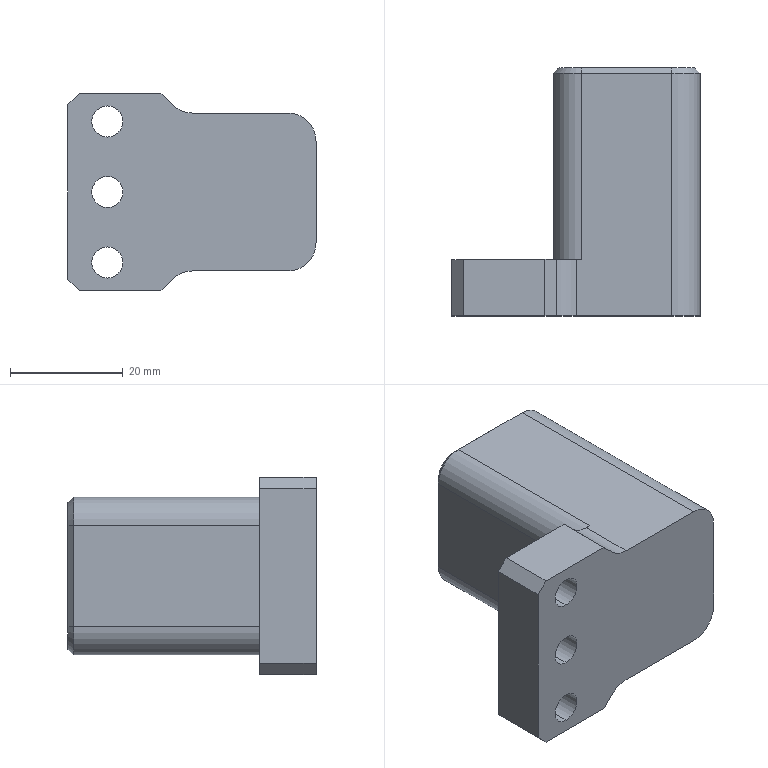Part | SolidWorks | features Chamfer 3, Fillet 2, HoleWzd 2, Extrusion 1, ICE 1 | 1 solid | 34 faces | box 44 x 44 x 35 mm | volume 36722 mm3 | plane 18 | cylinder 12 | cone 4 | commonest cylinder face diameters 5.5 x6 10 x6
STEP:
#1=CARTESIAN_POINT('',(-37.,0.,-15.25));
#2=VERTEX_POINT('',#1);
#3=CARTESIAN_POINT('',(-37.,0.,-9.75));
#4=VERTEX_POINT('',#3);
#5=CARTESIAN_POINT('',(-37.,0.,-12.5));
#6=DIRECTION('',(0.,1.,0.));
#7=DIRECTION('',(0.,0.,1.));
#8=AXIS2_PLACEMENT_3D('',#5,#6,#7);
#9=CIRCLE('',#8,2.75);
#10=EDGE_CURVE('',#2,#4,#9,.T.);
#11=ORIENTED_EDGE('',*,*,#10,.F.);
#12=CARTESIAN_POINT('',(-37.,10.,-15.25));
#13=VERTEX_POINT('',#12);
#14=CARTESIAN_POINT('',(-37.,10.,-15.25));
#15=DIRECTION('',(0.,1.,0.));
#16=VECTOR('',#15,1000.);
#17=LINE('',#14,#16);
#18=EDGE_CURVE('',#2,#13,#17,.T.);
#19=ORIENTED_EDGE('',*,*,#18,.T.);
#20=CARTESIAN_POINT('',(-37.,10.,-9.75));
#21=VERTEX_POINT('',#20);
#22=CARTESIAN_POINT('',(-37.,10.,-12.5));
#23=DIRECTION('',(0.,1.,0.));
#24=DIRECTION('',(0.,0.,1.));
#25=AXIS2_PLACEMENT_3D('',#22,#23,#24);
#26=CIRCLE('',#25,2.75);
#27=EDGE_CURVE('',#13,#21,#26,.T.);
#28=ORIENTED_EDGE('',*,*,#27,.T.);
#29=CARTESIAN_POINT('',(-37.,10.,-9.75));
#30=DIRECTION('',(0.,1.,0.));
#31=VECTOR('',#30,1000.);
#32=LINE('',#29,#31);
#33=EDGE_CURVE('',#4,#21,#32,.T.);
#34=ORIENTED_EDGE('',*,*,#33,.F.);
#35=EDGE_LOOP('',(#11,#19,#28,#34));
#36=FACE_OUTER_BOUND('',#35,.T.);
#37=CARTESIAN_POINT('',(-37.,10.,-12.5));
#38=DIRECTION('',(0.,1.,0.));
#39=DIRECTION('',(0.,0.,1.));
#40=AXIS2_PLACEMENT_3D('',#37,#38,#39);
#41=CYLINDRICAL_SURFACE('',#40,2.75);
#42=ADVANCED_FACE('',(#36),#41,.F.);
#43=CARTESIAN_POINT('',(-37.,0.,9.75));
#44=VERTEX_POINT('',#43);
#45=CARTESIAN_POINT('',(-37.,0.,15.25));
#46=VERTEX_POINT('',#45);
#47=CARTESIAN_POINT('',(-37.,0.,12.5));
#48=DIRECTION('',(0.,1.,0.));
#49=DIRECTION('',(0.,0.,1.));
#50=AXIS2_PLACEMENT_3D('',#47,#48,#49);
#51=CIRCLE('',#50,2.75);
#52=EDGE_CURVE('',#44,#46,#51,.T.);
#53=ORIENTED_EDGE('',*,*,#52,.F.);
#54=CARTESIAN_POINT('',(-37.,10.,9.75));
#55=VERTEX_POINT('',#54);
#56=CARTESIAN_POINT('',(-37.,10.,9.75));
#57=DIRECTION('',(0.,1.,0.));
#58=VECTOR('',#57,1000.);
#59=LINE('',#56,#58);
#60=EDGE_CURVE('',#44,#55,#59,.T.);
#61=ORIENTED_EDGE('',*,*,#60,.T.);
#62=CARTESIAN_POINT('',(-37.,10.,15.25));
#63=VERTEX_POINT('',#62);
#64=CARTESIAN_POINT('',(-37.,10.,12.5));
#65=DIRECTION('',(0.,1.,0.));
#66=DIRECTION('',(0.,0.,1.));
#67=AXIS2_PLACEMENT_3D('',#64,#65,#66);
#68=CIRCLE('',#67,2.75);
#69=EDGE_CURVE('',#55,#63,#68,.T.);
#70=ORIENTED_EDGE('',*,*,#69,.T.);
#71=CARTESIAN_POINT('',(-37.,10.,15.25));
#72=DIRECTION('',(0.,1.,0.));
#73=VECTOR('',#72,1000.);
#74=LINE('',#71,#73);
#75=EDGE_CURVE('',#46,#63,#74,.T.);
#76=ORIENTED_EDGE('',*,*,#75,.F.);
#77=EDGE_LOOP('',(#53,#61,#70,#76));
#78=FACE_OUTER_BOUND('',#77,.T.);
#79=CARTESIAN_POINT('',(-37.,10.,12.5));
#80=DIRECTION('',(0.,1.,0.));
#81=DIRECTION('',(0.,0.,1.));
#82=AXIS2_PLACEMENT_3D('',#79,#80,#81);
#83=CYLINDRICAL_SURFACE('',#82,2.75);
#84=ADVANCED_FACE('',(#78),#83,.F.);
#85=CARTESIAN_POINT('',(-37.,0.,-2.75));
#86=VERTEX_POINT('',#85);
#87=CARTESIAN_POINT('',(-37.,0.,2.75));
#88=VERTEX_POINT('',#87);
#89=CARTESIAN_POINT('',(-37.,0.,0.));
#90=DIRECTION('',(0.,1.,0.));
#91=DIRECTION('',(0.,0.,1.));
#92=AXIS2_PLACEMENT_3D('',#89,#90,#91);
#93=CIRCLE('',#92,2.75);
#94=EDGE_CURVE('',#86,#88,#93,.T.);
#95=ORIENTED_EDGE('',*,*,#94,.F.);
#96=CARTESIAN_POINT('',(-37.,10.,-2.75));
#97=VERTEX_POINT('',#96);
#98=CARTESIAN_POINT('',(-37.,10.,-2.75));
#99=DIRECTION('',(0.,1.,0.));
#100=VECTOR('',#99,1000.);
#101=LINE('',#98,#100);
#102=EDGE_CURVE('',#86,#97,#101,.T.);
#103=ORIENTED_EDGE('',*,*,#102,.T.);
#104=CARTESIAN_POINT('',(-37.,10.,2.75));
#105=VERTEX_POINT('',#104);
#106=CARTESIAN_POINT('',(-37.,10.,0.));
#107=DIRECTION('',(0.,1.,0.));
#108=DIRECTION('',(0.,0.,1.));
#109=AXIS2_PLACEMENT_3D('',#106,#107,#108);
#110=CIRCLE('',#109,2.75);
#111=EDGE_CURVE('',#97,#105,#110,.T.);
#112=ORIENTED_EDGE('',*,*,#111,.T.);
#113=CARTESIAN_POINT('',(-37.,10.,2.75));
#114=DIRECTION('',(0.,1.,0.));
#115=VECTOR('',#114,1000.);
#116=LINE('',#113,#115);
#117=EDGE_CURVE('',#88,#105,#116,.T.);
#118=ORIENTED_EDGE('',*,*,#117,.F.);
#119=EDGE_LOOP('',(#95,#103,#112,#118));
#120=FACE_OUTER_BOUND('',#119,.T.);
#121=CARTESIAN_POINT('',(-37.,10.,0.));
#122=DIRECTION('',(0.,1.,0.));
#123=DIRECTION('',(0.,0.,1.));
#124=AXIS2_PLACEMENT_3D('',#121,#122,#123);
#125=CYLINDRICAL_SURFACE('',#124,2.75);
#126=ADVANCED_FACE('',(#120),#125,.F.);
#127=CARTESIAN_POINT('',(-37.,0.,-12.5));
#128=DIRECTION('',(0.,1.,0.));
#129=DIRECTION('',(0.,0.,1.));
#130=AXIS2_PLACEMENT_3D('',#127,#128,#129);
#131=CIRCLE('',#130,2.75);
#132=EDGE_CURVE('',#4,#2,#131,.T.);
#133=ORIENTED_EDGE('',*,*,#132,.T.);
#134=ORIENTED_EDGE('',*,*,#10,.T.);
#135=EDGE_LOOP('',(#133,#134));
#136=FACE_BOUND('',#135,.T.);
#137=CARTESIAN_POINT('',(-37.,0.,12.5));
#138=DIRECTION('',(0.,1.,0.));
#139=DIRECTION('',(0.,0.,1.));
#140=AXIS2_PLACEMENT_3D('',#137,#138,#139);
#141=CIRCLE('',#140,2.75);
#142=EDGE_CURVE('',#46,#44,#141,.T.);
#143=ORIENTED_EDGE('',*,*,#142,.T.);
#144=ORIENTED_EDGE('',*,*,#52,.T.);
#145=EDGE_LOOP('',(#143,#144));
#146=FACE_BOUND('',#145,.T.);
#147=CARTESIAN_POINT('',(-37.,0.,0.));
#148=DIRECTION('',(0.,1.,0.));
#149=DIRECTION('',(0.,0.,1.));
#150=AXIS2_PLACEMENT_3D('',#147,#148,#149);
#151=CIRCLE('',#150,2.75);
#152=EDGE_CURVE('',#88,#86,#151,.T.);
#153=ORIENTED_EDGE('',*,*,#152,.T.);
#154=ORIENTED_EDGE('',*,*,#94,.T.);
#155=EDGE_LOOP('',(#153,#154));
#156=FACE_BOUND('',#155,.T.);
#157=CARTESIAN_POINT('',(-44.,0.,15.5));
#158=VERTEX_POINT('',#157);
#159=CARTESIAN_POINT('',(-44.,0.,-15.5));
#160=VERTEX_POINT('',#159);
#161=CARTESIAN_POINT('',(-44.,0.,14.));
#162=DIRECTION('',(0.,0.,-1.));
#163=VECTOR('',#162,1000.);
#164=LINE('',#161,#163);
#165=EDGE_CURVE('',#158,#160,#164,.T.);
#166=ORIENTED_EDGE('',*,*,#165,.T.);
#167=CARTESIAN_POINT('',(-42.,0.,-17.5));
#168=VERTEX_POINT('',#167);
#169=CARTESIAN_POINT('',(-44.,0.,-15.5));
#170=DIRECTION('',(0.7071,0.,-0.7071));
#171=VECTOR('',#170,1000.);
#172=LINE('',#169,#171);
#173=EDGE_CURVE('',#160,#168,#172,.T.);
#174=ORIENTED_EDGE('',*,*,#173,.T.);
#175=CARTESIAN_POINT('',(-27.5,0.,-17.5));
#176=VERTEX_POINT('',#175);
#177=CARTESIAN_POINT('',(-44.,0.,-17.5));
#178=DIRECTION('',(1.,0.,0.));
#179=VECTOR('',#178,1000.);
#180=LINE('',#177,#179);
#181=EDGE_CURVE('',#168,#176,#180,.T.);
#182=ORIENTED_EDGE('',*,*,#181,.T.);
#183=CARTESIAN_POINT('',(-25.464,0.,-15.464));
#184=VERTEX_POINT('',#183);
#185=CARTESIAN_POINT('',(-27.5,0.,-17.5));
#186=DIRECTION('',(0.7071,0.,0.7071));
#187=VECTOR('',#186,1000.);
#188=LINE('',#185,#187);
#189=EDGE_CURVE('',#176,#184,#188,.T.);
#190=ORIENTED_EDGE('',*,*,#189,.T.);
#191=CARTESIAN_POINT('',(-21.929,0.,-14.));
#192=VERTEX_POINT('',#191);
#193=CARTESIAN_POINT('',(-21.929,0.,-19.));
#194=DIRECTION('',(0.,1.,0.));
#195=DIRECTION('',(0.,0.,1.));
#196=AXIS2_PLACEMENT_3D('',#193,#194,#195);
#197=CIRCLE('',#196,5.);
#198=EDGE_CURVE('',#184,#192,#197,.T.);
#199=ORIENTED_EDGE('',*,*,#198,.T.);
#200=CARTESIAN_POINT('',(-5.,0.,-14.));
#201=VERTEX_POINT('',#200);
#202=CARTESIAN_POINT('',(-44.,0.,-14.));
#203=DIRECTION('',(1.,0.,0.));
#204=VECTOR('',#203,1000.);
#205=LINE('',#202,#204);
#206=EDGE_CURVE('',#192,#201,#205,.T.);
#207=ORIENTED_EDGE('',*,*,#206,.T.);
#208=CARTESIAN_POINT('',(0.,0.,-9.));
#209=VERTEX_POINT('',#208);
#210=CARTESIAN_POINT('',(-5.,0.,-9.));
#211=DIRECTION('',(0.,-1.,0.));
#212=DIRECTION('',(0.,0.,1.));
#213=AXIS2_PLACEMENT_3D('',#210,#211,#212);
#214=CIRCLE('',#213,5.);
#215=EDGE_CURVE('',#201,#209,#214,.T.);
#216=ORIENTED_EDGE('',*,*,#215,.T.);
#217=CARTESIAN_POINT('',(0.,0.,9.));
#218=VERTEX_POINT('',#217);
#219=CARTESIAN_POINT('',(0.,0.,14.));
#220=DIRECTION('',(0.,0.,-1.));
#221=VECTOR('',#220,1000.);
#222=LINE('',#219,#221);
#223=EDGE_CURVE('',#218,#209,#222,.T.);
#224=ORIENTED_EDGE('',*,*,#223,.F.);
#225=CARTESIAN_POINT('',(-5.,0.,14.));
#226=VERTEX_POINT('',#225);
#227=CARTESIAN_POINT('',(-5.,0.,9.));
#228=DIRECTION('',(0.,-1.,0.));
#229=DIRECTION('',(0.,0.,1.));
#230=AXIS2_PLACEMENT_3D('',#227,#228,#229);
#231=CIRCLE('',#230,5.);
#232=EDGE_CURVE('',#218,#226,#231,.T.);
#233=ORIENTED_EDGE('',*,*,#232,.T.);
#234=CARTESIAN_POINT('',(-21.929,0.,14.));
#235=VERTEX_POINT('',#234);
#236=CARTESIAN_POINT('',(-44.,0.,14.));
#237=DIRECTION('',(1.,0.,0.));
#238=VECTOR('',#237,1000.);
#239=LINE('',#236,#238);
#240=EDGE_CURVE('',#235,#226,#239,.T.);
#241=ORIENTED_EDGE('',*,*,#240,.F.);
#242=CARTESIAN_POINT('',(-25.464,0.,15.464));
#243=VERTEX_POINT('',#242);
#244=CARTESIAN_POINT('',(-21.929,0.,19.));
#245=DIRECTION('',(0.,1.,0.));
#246=DIRECTION('',(0.,0.,1.));
#247=AXIS2_PLACEMENT_3D('',#244,#245,#246);
#248=CIRCLE('',#247,5.);
#249=EDGE_CURVE('',#235,#243,#248,.T.);
#250=ORIENTED_EDGE('',*,*,#249,.T.);
#251=CARTESIAN_POINT('',(-27.5,0.,17.5));
#252=VERTEX_POINT('',#251);
#253=CARTESIAN_POINT('',(-24.,0.,14.));
#254=DIRECTION('',(-0.7071,0.,0.7071));
#255=VECTOR('',#254,1000.);
#256=LINE('',#253,#255);
#257=EDGE_CURVE('',#243,#252,#256,.T.);
#258=ORIENTED_EDGE('',*,*,#257,.T.);
#259=CARTESIAN_POINT('',(-42.,0.,17.5));
#260=VERTEX_POINT('',#259);
#261=CARTESIAN_POINT('',(-44.,0.,17.5));
#262=DIRECTION('',(-1.,0.,0.));
#263=VECTOR('',#262,1000.);
#264=LINE('',#261,#263);
#265=EDGE_CURVE('',#252,#260,#264,.T.);
#266=ORIENTED_EDGE('',*,*,#265,.T.);
#267=CARTESIAN_POINT('',(-42.,0.,17.5));
#268=DIRECTION('',(-0.7071,0.,-0.7071));
#269=VECTOR('',#268,1000.);
#270=LINE('',#267,#269);
#271=EDGE_CURVE('',#260,#158,#270,.T.);
#272=ORIENTED_EDGE('',*,*,#271,.T.);
#273=EDGE_LOOP('',(#166,#174,#182,#190,#199,#207,#216,#224,#233,#241,#250,#258,#266,#272));
#274=FACE_OUTER_BOUND('',#273,.T.);
#275=CARTESIAN_POINT('',(-44.,0.,14.));
#276=DIRECTION('',(0.,1.,0.));
#277=DIRECTION('',(0.,0.,1.));
#278=AXIS2_PLACEMENT_3D('',#275,#276,#277);
#279=PLANE('',#278);
#280=ADVANCED_FACE('',(#136,#146,#156,#274),#279,.F.);
#281=CARTESIAN_POINT('',(0.,43.,-9.));
#282=VERTEX_POINT('',#281);
#283=CARTESIAN_POINT('',(0.,0.,-9.));
#284=DIRECTION('',(0.,1.,0.));
#285=VECTOR('',#284,1000.);
#286=LINE('',#283,#285);
#287=EDGE_CURVE('',#209,#282,#286,.T.);
#288=ORIENTED_EDGE('',*,*,#287,.T.);
#289=CARTESIAN_POINT('',(0.,43.,9.));
#290=VERTEX_POINT('',#289);
#291=CARTESIAN_POINT('',(0.,43.,14.));
#292=DIRECTION('',(0.,0.,1.));
#293=VECTOR('',#292,1000.);
#294=LINE('',#291,#293);
#295=EDGE_CURVE('',#282,#290,#294,.T.);
#296=ORIENTED_EDGE('',*,*,#295,.T.);
#297=CARTESIAN_POINT('',(0.,0.,9.));
#298=DIRECTION('',(0.,-1.,0.));
#299=VECTOR('',#298,1000.);
#300=LINE('',#297,#299);
#301=EDGE_CURVE('',#290,#218,#300,.T.);
#302=ORIENTED_EDGE('',*,*,#301,.T.);
#303=ORIENTED_EDGE('',*,*,#223,.T.);
#304=EDGE_LOOP('',(#288,#296,#302,#303));
#305=FACE_OUTER_BOUND('',#304,.T.);
#306=CARTESIAN_POINT('',(0.,0.,14.));
#307=DIRECTION('',(-1.,0.,0.));
#308=DIRECTION('',(0.,0.,1.));
#309=AXIS2_PLACEMENT_3D('',#306,#307,#308);
#310=PLANE('',#309);
#311=ADVANCED_FACE('',(#305),#310,.F.);
#312=CARTESIAN_POINT('',(-1.,44.,9.));
#313=VERTEX_POINT('',#312);
#314=CARTESIAN_POINT('',(-1.,44.,-9.));
#315=VERTEX_POINT('',#314);
#316=CARTESIAN_POINT('',(-1.,44.,14.));
#317=DIRECTION('',(0.,0.,-1.));
#318=VECTOR('',#317,1000.);
#319=LINE('',#316,#318);
#320=EDGE_CURVE('',#313,#315,#319,.T.);
#321=ORIENTED_EDGE('',*,*,#320,.T.);
#322=CARTESIAN_POINT('',(-5.,44.,-13.));
#323=VERTEX_POINT('',#322);
#324=CARTESIAN_POINT('',(-5.,44.,-9.));
#325=DIRECTION('',(0.,1.,0.));
#326=DIRECTION('',(1.,0.,0.));
#327=AXIS2_PLACEMENT_3D('',#324,#325,#326);
#328=CIRCLE('',#327,4.);
#329=EDGE_CURVE('',#315,#323,#328,.T.);
#330=ORIENTED_EDGE('',*,*,#329,.T.);
#331=CARTESIAN_POINT('',(-21.,44.,-13.));
#332=VERTEX_POINT('',#331);
#333=CARTESIAN_POINT('',(0.,44.,-13.));
#334=DIRECTION('',(-1.,0.,0.));
#335=VECTOR('',#334,1000.);
#336=LINE('',#333,#335);
#337=EDGE_CURVE('',#323,#332,#336,.T.);
#338=ORIENTED_EDGE('',*,*,#337,.T.);
#339=CARTESIAN_POINT('',(-25.,44.,-9.));
#340=VERTEX_POINT('',#339);
#341=CARTESIAN_POINT('',(-21.,44.,-9.));
#342=DIRECTION('',(0.,1.,0.));
#343=DIRECTION('',(1.,0.,0.));
#344=AXIS2_PLACEMENT_3D('',#341,#342,#343);
#345=CIRCLE('',#344,4.);
#346=EDGE_CURVE('',#332,#340,#345,.T.);
#347=ORIENTED_EDGE('',*,*,#346,.T.);
#348=CARTESIAN_POINT('',(-25.,44.,9.));
#349=VERTEX_POINT('',#348);
#350=CARTESIAN_POINT('',(-25.,44.,14.));
#351=DIRECTION('',(0.,0.,1.));
#352=VECTOR('',#351,1000.);
#353=LINE('',#350,#352);
#354=EDGE_CURVE('',#340,#349,#353,.T.);
#355=ORIENTED_EDGE('',*,*,#354,.T.);
#356=CARTESIAN_POINT('',(-21.,44.,13.));
#357=VERTEX_POINT('',#356);
#358=CARTESIAN_POINT('',(-21.,44.,9.));
#359=DIRECTION('',(0.,1.,0.));
#360=DIRECTION('',(1.,0.,0.));
#361=AXIS2_PLACEMENT_3D('',#358,#359,#360);
#362=CIRCLE('',#361,4.);
#363=EDGE_CURVE('',#349,#357,#362,.T.);
#364=ORIENTED_EDGE('',*,*,#363,.T.);
#365=CARTESIAN_POINT('',(-5.,44.,13.));
#366=VERTEX_POINT('',#365);
#367=CARTESIAN_POINT('',(-5.,44.,13.));
#368=DIRECTION('',(1.,0.,0.));
#369=VECTOR('',#368,1000.);
#370=LINE('',#367,#369);
#371=EDGE_CURVE('',#357,#366,#370,.T.);
#372=ORIENTED_EDGE('',*,*,#371,.T.);
#373=CARTESIAN_POINT('',(-5.,44.,9.));
#374=DIRECTION('',(0.,1.,0.));
#375=DIRECTION('',(1.,0.,0.));
#376=AXIS2_PLACEMENT_3D('',#373,#374,#375);
#377=CIRCLE('',#376,4.);
#378=EDGE_CURVE('',#366,#313,#377,.T.);
#379=ORIENTED_EDGE('',*,*,#378,.T.);
#380=EDGE_LOOP('',(#321,#330,#338,#347,#355,#364,#372,#379));
#381=FACE_OUTER_BOUND('',#380,.T.);
#382=CARTESIAN_POINT('',(0.,44.,14.));
#383=DIRECTION('',(0.,-1.,0.));
#384=DIRECTION('',(1.,0.,0.));
#385=AXIS2_PLACEMENT_3D('',#382,#383,#384);
#386=PLANE('',#385);
#387=ADVANCED_FACE('',(#381),#386,.F.);
#388=CARTESIAN_POINT('',(-26.,10.,9.));
#389=VERTEX_POINT('',#388);
#390=CARTESIAN_POINT('',(-26.,43.,9.));
#391=VERTEX_POINT('',#390);
#392=CARTESIAN_POINT('',(-26.,44.,9.));
#393=DIRECTION('',(0.,1.,0.));
#394=VECTOR('',#393,1000.);
#395=LINE('',#392,#394);
#396=EDGE_CURVE('',#389,#391,#395,.T.);
#397=ORIENTED_EDGE('',*,*,#396,.T.);
#398=CARTESIAN_POINT('',(-26.,43.,-9.));
#399=VERTEX_POINT('',#398);
#400=CARTESIAN_POINT('',(-26.,43.,14.));
#401=DIRECTION('',(0.,0.,-1.));
#402=VECTOR('',#401,1000.);
#403=LINE('',#400,#402);
#404=EDGE_CURVE('',#391,#399,#403,.T.);
#405=ORIENTED_EDGE('',*,*,#404,.T.);
#406=CARTESIAN_POINT('',(-26.,10.,-9.));
#407=VERTEX_POINT('',#406);
#408=CARTESIAN_POINT('',(-26.,44.,-9.));
#409=DIRECTION('',(0.,-1.,0.));
#410=VECTOR('',#409,1000.);
#411=LINE('',#408,#410);
#412=EDGE_CURVE('',#399,#407,#411,.T.);
#413=ORIENTED_EDGE('',*,*,#412,.T.);
#414=CARTESIAN_POINT('',(-26.,10.,14.));
#415=DIRECTION('',(0.,0.,-1.));
#416=VECTOR('',#415,1000.);
#417=LINE('',#414,#416);
#418=EDGE_CURVE('',#389,#407,#417,.T.);
#419=ORIENTED_EDGE('',*,*,#418,.F.);
#420=EDGE_LOOP('',(#397,#405,#413,#419));
#421=FACE_OUTER_BOUND('',#420,.T.);
#422=CARTESIAN_POINT('',(-26.,44.,14.));
#423=DIRECTION('',(1.,0.,0.));
#424=DIRECTION('',(0.,1.,0.));
#425=AXIS2_PLACEMENT_3D('',#422,#423,#424);
#426=PLANE('',#425);
#427=ADVANCED_FACE('',(#421),#426,.F.);
#428=CARTESIAN_POINT('',(-37.,10.,-12.5));
#429=DIRECTION('',(0.,1.,0.));
#430=DIRECTION('',(0.,0.,1.));
#431=AXIS2_PLACEMENT_3D('',#428,#429,#430);
#432=CIRCLE('',#431,2.75);
#433=EDGE_CURVE('',#21,#13,#432,.T.);
#434=ORIENTED_EDGE('',*,*,#433,.F.);
#435=ORIENTED_EDGE('',*,*,#27,.F.);
#436=EDGE_LOOP('',(#434,#435));
#437=FACE_BOUND('',#436,.T.);
#438=CARTESIAN_POINT('',(-37.,10.,12.5));
#439=DIRECTION('',(0.,1.,0.));
#440=DIRECTION('',(0.,0.,1.));
#441=AXIS2_PLACEMENT_3D('',#438,#439,#440);
#442=CIRCLE('',#441,2.75);
#443=EDGE_CURVE('',#63,#55,#442,.T.);
#444=ORIENTED_EDGE('',*,*,#443,.F.);
#445=ORIENTED_EDGE('',*,*,#69,.F.);
#446=EDGE_LOOP('',(#444,#445));
#447=FACE_BOUND('',#446,.T.);
#448=CARTESIAN_POINT('',(-37.,10.,0.));
#449=DIRECTION('',(0.,1.,0.));
#450=DIRECTION('',(0.,0.,1.));
#451=AXIS2_PLACEMENT_3D('',#448,#449,#450);
#452=CIRCLE('',#451,2.75);
#453=EDGE_CURVE('',#105,#97,#452,.T.);
#454=ORIENTED_EDGE('',*,*,#453,.F.);
#455=ORIENTED_EDGE('',*,*,#111,.F.);
#456=EDGE_LOOP('',(#454,#455));
#457=FACE_BOUND('',#456,.T.);
#458=CARTESIAN_POINT('',(-27.5,10.,-17.5));
#459=VERTEX_POINT('',#458);
#460=CARTESIAN_POINT('',(-42.,10.,-17.5));
#461=VERTEX_POINT('',#460);
#462=CARTESIAN_POINT('',(-44.,10.,-17.5));
#463=DIRECTION('',(-1.,0.,0.));
#464=VECTOR('',#463,1000.);
#465=LINE('',#462,#464);
#466=EDGE_CURVE('',#459,#461,#465,.T.);
#467=ORIENTED_EDGE('',*,*,#466,.T.);
#468=CARTESIAN_POINT('',(-44.,10.,-15.5));
#469=VERTEX_POINT('',#468);
#470=CARTESIAN_POINT('',(-44.,10.,-15.5));
#471=DIRECTION('',(-0.7071,0.,0.7071));
#472=VECTOR('',#471,1000.);
#473=LINE('',#470,#472);
#474=EDGE_CURVE('',#461,#469,#473,.T.);
#475=ORIENTED_EDGE('',*,*,#474,.T.);
#476=CARTESIAN_POINT('',(-44.,10.,15.5));
#477=VERTEX_POINT('',#476);
#478=CARTESIAN_POINT('',(-44.,10.,14.));
#479=DIRECTION('',(0.,0.,-1.));
#480=VECTOR('',#479,1000.);
#481=LINE('',#478,#480);
#482=EDGE_CURVE('',#477,#469,#481,.T.);
#483=ORIENTED_EDGE('',*,*,#482,.F.);
#484=CARTESIAN_POINT('',(-42.,10.,17.5));
#485=VERTEX_POINT('',#484);
#486=CARTESIAN_POINT('',(-42.,10.,17.5));
#487=DIRECTION('',(0.7071,0.,0.7071));
#488=VECTOR('',#487,1000.);
#489=LINE('',#486,#488);
#490=EDGE_CURVE('',#477,#485,#489,.T.);
#491=ORIENTED_EDGE('',*,*,#490,.T.);
#492=CARTESIAN_POINT('',(-27.5,10.,17.5));
#493=VERTEX_POINT('',#492);
#494=CARTESIAN_POINT('',(-44.,10.,17.5));
#495=DIRECTION('',(1.,0.,0.));
#496=VECTOR('',#495,1000.);
#497=LINE('',#494,#496);
#498=EDGE_CURVE('',#485,#493,#497,.T.);
#499=ORIENTED_EDGE('',*,*,#498,.T.);
#500=CARTESIAN_POINT('',(-25.464,10.,15.464));
#501=VERTEX_POINT('',#500);
#502=CARTESIAN_POINT('',(-24.,10.,14.));
#503=DIRECTION('',(0.7071,0.,-0.7071));
#504=VECTOR('',#503,1000.);
#505=LINE('',#502,#504);
#506=EDGE_CURVE('',#493,#501,#505,.T.);
#507=ORIENTED_EDGE('',*,*,#506,.T.);
#508=CARTESIAN_POINT('',(-21.929,10.,14.));
#509=VERTEX_POINT('',#508);
#510=CARTESIAN_POINT('',(-21.929,10.,19.));
#511=DIRECTION('',(0.,-1.,0.));
#512=DIRECTION('',(1.,0.,0.));
#513=AXIS2_PLACEMENT_3D('',#510,#511,#512);
#514=CIRCLE('',#513,5.);
#515=EDGE_CURVE('',#501,#509,#514,.T.);
#516=ORIENTED_EDGE('',*,*,#515,.T.);
#517=CARTESIAN_POINT('',(-21.,10.,14.));
#518=VERTEX_POINT('',#517);
#519=CARTESIAN_POINT('',(-26.,10.,14.));
#520=DIRECTION('',(-1.,0.,0.));
#521=VECTOR('',#520,1000.);
#522=LINE('',#519,#521);
#523=EDGE_CURVE('',#518,#509,#522,.T.);
#524=ORIENTED_EDGE('',*,*,#523,.F.);
#525=CARTESIAN_POINT('',(-21.,10.,9.));
#526=DIRECTION('',(0.,-1.,0.));
#527=DIRECTION('',(1.,0.,0.));
#528=AXIS2_PLACEMENT_3D('',#525,#526,#527);
#529=CIRCLE('',#528,5.);
#530=EDGE_CURVE('',#518,#389,#529,.T.);
#531=ORIENTED_EDGE('',*,*,#530,.T.);
#532=ORIENTED_EDGE('',*,*,#418,.T.);
#533=CARTESIAN_POINT('',(-21.,10.,-14.));
#534=VERTEX_POINT('',#533);
#535=CARTESIAN_POINT('',(-21.,10.,-9.));
#536=DIRECTION('',(0.,-1.,0.));
#537=DIRECTION('',(1.,0.,0.));
#538=AXIS2_PLACEMENT_3D('',#535,#536,#537);
#539=CIRCLE('',#538,5.);
#540=EDGE_CURVE('',#407,#534,#539,.T.);
#541=ORIENTED_EDGE('',*,*,#540,.T.);
#542=CARTESIAN_POINT('',(-21.929,10.,-14.));
#543=VERTEX_POINT('',#542);
#544=CARTESIAN_POINT('',(-26.,10.,-14.));
#545=DIRECTION('',(-1.,0.,0.));
#546=VECTOR('',#545,1000.);
#547=LINE('',#544,#546);
#548=EDGE_CURVE('',#534,#543,#547,.T.);
#549=ORIENTED_EDGE('',*,*,#548,.T.);
#550=CARTESIAN_POINT('',(-25.464,10.,-15.464));
#551=VERTEX_POINT('',#550);
#552=CARTESIAN_POINT('',(-21.929,10.,-19.));
#553=DIRECTION('',(0.,-1.,0.));
#554=DIRECTION('',(1.,0.,0.));
#555=AXIS2_PLACEMENT_3D('',#552,#553,#554);
#556=CIRCLE('',#555,5.);
#557=EDGE_CURVE('',#543,#551,#556,.T.);
#558=ORIENTED_EDGE('',*,*,#557,.T.);
#559=CARTESIAN_POINT('',(-27.5,10.,-17.5));
#560=DIRECTION('',(-0.7071,0.,-0.7071));
#561=VECTOR('',#560,1000.);
#562=LINE('',#559,#561);
#563=EDGE_CURVE('',#551,#459,#562,.T.);
#564=ORIENTED_EDGE('',*,*,#563,.T.);
#565=EDGE_LOOP('',(#467,#475,#483,#491,#499,#507,#516,#524,#531,#532,#541,#549,#558,#564));
#566=FACE_OUTER_BOUND('',#565,.T.);
#567=CARTESIAN_POINT('',(-26.,10.,14.));
#568=DIRECTION('',(0.,-1.,0.));
#569=DIRECTION('',(1.,0.,0.));
#570=AXIS2_PLACEMENT_3D('',#567,#568,#569);
#571=PLANE('',#570);
#572=ADVANCED_FACE('',(#437,#447,#457,#566),#571,.F.);
#573=ORIENTED_EDGE('',*,*,#482,.T.);
#574=CARTESIAN_POINT('',(-44.,0.,-15.5));
#575=DIRECTION('',(0.,-1.,0.));
#576=VECTOR('',#575,1000.);
#577=LINE('',#574,#576);
#578=EDGE_CURVE('',#469,#160,#577,.T.);
#579=ORIENTED_EDGE('',*,*,#578,.T.);
#580=ORIENTED_EDGE('',*,*,#165,.F.);
#581=CARTESIAN_POINT('',(-44.,10.,15.5));
#582=DIRECTION('',(0.,1.,0.));
#583=VECTOR('',#582,1000.);
#584=LINE('',#581,#583);
#585=EDGE_CURVE('',#158,#477,#584,.T.);
#586=ORIENTED_EDGE('',*,*,#585,.T.);
#587=EDGE_LOOP('',(#573,#579,#580,#586));
#588=FACE_OUTER_BOUND('',#587,.T.);
#589=CARTESIAN_POINT('',(-44.,10.,14.));
#590=DIRECTION('',(1.,0.,0.));
#591=DIRECTION('',(0.,0.,-1.));
#592=AXIS2_PLACEMENT_3D('',#589,#590,#591);
#593=PLANE('',#592);
#594=ADVANCED_FACE('',(#588),#593,.F.);
#595=ORIENTED_EDGE('',*,*,#523,.T.);
#596=CARTESIAN_POINT('',(-21.929,0.,14.));
#597=DIRECTION('',(0.,-1.,0.));
#598=VECTOR('',#597,1000.);
#599=LINE('',#596,#598);
#600=EDGE_CURVE('',#509,#235,#599,.T.);
#601=ORIENTED_EDGE('',*,*,#600,.T.);
#602=ORIENTED_EDGE('',*,*,#240,.T.);
#603=CARTESIAN_POINT('',(-5.,43.,14.));
#604=VERTEX_POINT('',#603);
#605=CARTESIAN_POINT('',(-5.,44.,14.));
#606=DIRECTION('',(0.,1.,0.));
#607=VECTOR('',#606,1000.);
#608=LINE('',#605,#607);
#609=EDGE_CURVE('',#226,#604,#608,.T.);
#610=ORIENTED_EDGE('',*,*,#609,.T.);
#611=CARTESIAN_POINT('',(-21.,43.,14.));
#612=VERTEX_POINT('',#611);
#613=CARTESIAN_POINT('',(-21.,43.,14.));
#614=DIRECTION('',(-1.,0.,0.));
#615=VECTOR('',#614,1000.);
#616=LINE('',#613,#615);
#617=EDGE_CURVE('',#604,#612,#616,.T.);
#618=ORIENTED_EDGE('',*,*,#617,.T.);
#619=CARTESIAN_POINT('',(-21.,10.,14.));
#620=DIRECTION('',(0.,-1.,0.));
#621=VECTOR('',#620,1000.);
#622=LINE('',#619,#621);
#623=EDGE_CURVE('',#612,#518,#622,.T.);
#624=ORIENTED_EDGE('',*,*,#623,.T.);
#625=EDGE_LOOP('',(#595,#601,#602,#610,#618,#624));
#626=FACE_OUTER_BOUND('',#625,.T.);
#627=CARTESIAN_POINT('',(0.,0.,14.));
#628=DIRECTION('',(0.,0.,1.));
#629=DIRECTION('',(1.,0.,0.));
#630=AXIS2_PLACEMENT_3D('',#627,#628,#629);
#631=PLANE('',#630);
#632=ADVANCED_FACE('',(#626),#631,.T.);
#633=ORIENTED_EDGE('',*,*,#206,.F.);
#634=CARTESIAN_POINT('',(-21.929,0.,-14.));
#635=DIRECTION('',(0.,1.,0.));
#636=VECTOR('',#635,1000.);
#637=LINE('',#634,#636);
#638=EDGE_CURVE('',#192,#543,#637,.T.);
#639=ORIENTED_EDGE('',*,*,#638,.T.);
#640=ORIENTED_EDGE('',*,*,#548,.F.);
#641=CARTESIAN_POINT('',(-21.,43.,-14.));
#642=VERTEX_POINT('',#641);
#643=CARTESIAN_POINT('',(-21.,0.,-14.));
#644=DIRECTION('',(0.,1.,0.));
#645=VECTOR('',#644,1000.);
#646=LINE('',#643,#645);
#647=EDGE_CURVE('',#534,#642,#646,.T.);
#648=ORIENTED_EDGE('',*,*,#647,.T.);
#649=CARTESIAN_POINT('',(-5.,43.,-14.));
#650=VERTEX_POINT('',#649);
#651=CARTESIAN_POINT('',(0.,43.,-14.));
#652=DIRECTION('',(1.,0.,0.));
#653=VECTOR('',#652,1000.);
#654=LINE('',#651,#653);
#655=EDGE_CURVE('',#642,#650,#654,.T.);
#656=ORIENTED_EDGE('',*,*,#655,.T.);
#657=CARTESIAN_POINT('',(-5.,0.,-14.));
#658=DIRECTION('',(0.,-1.,0.));
#659=VECTOR('',#658,1000.);
#660=LINE('',#657,#659);
#661=EDGE_CURVE('',#650,#201,#660,.T.);
#662=ORIENTED_EDGE('',*,*,#661,.T.);
#663=EDGE_LOOP('',(#633,#639,#640,#648,#656,#662));
#664=FACE_OUTER_BOUND('',#663,.T.);
#665=CARTESIAN_POINT('',(0.,0.,-14.));
#666=DIRECTION('',(0.,0.,1.));
#667=DIRECTION('',(1.,0.,0.));
#668=AXIS2_PLACEMENT_3D('',#665,#666,#667);
#669=PLANE('',#668);
#670=ADVANCED_FACE('',(#664),#669,.F.);
#671=ORIENTED_EDGE('',*,*,#102,.F.);
#672=ORIENTED_EDGE('',*,*,#152,.F.);
#673=ORIENTED_EDGE('',*,*,#117,.T.);
#674=ORIENTED_EDGE('',*,*,#453,.T.);
#675=EDGE_LOOP('',(#671,#672,#673,#674));
#676=FACE_OUTER_BOUND('',#675,.T.);
#677=CARTESIAN_POINT('',(-37.,10.,0.));
#678=DIRECTION('',(0.,1.,0.));
#679=DIRECTION('',(0.,0.,1.));
#680=AXIS2_PLACEMENT_3D('',#677,#678,#679);
#681=CYLINDRICAL_SURFACE('',#680,2.75);
#682=ADVANCED_FACE('',(#676),#681,.F.);
#683=ORIENTED_EDGE('',*,*,#412,.F.);
#684=CARTESIAN_POINT('',(-21.,43.,-9.));
#685=DIRECTION('',(0.,-1.,0.));
#686=DIRECTION('',(0.,0.,-1.));
#687=AXIS2_PLACEMENT_3D('',#684,#685,#686);
#688=CIRCLE('',#687,5.);
#689=EDGE_CURVE('',#399,#642,#688,.T.);
#690=ORIENTED_EDGE('',*,*,#689,.T.);
#691=ORIENTED_EDGE('',*,*,#647,.F.);
#692=ORIENTED_EDGE('',*,*,#540,.F.);
#693=EDGE_LOOP('',(#683,#690,#691,#692));
#694=FACE_OUTER_BOUND('',#693,.T.);
#695=CARTESIAN_POINT('',(-21.,44.,-9.));
#696=DIRECTION('',(0.,-1.,0.));
#697=DIRECTION('',(1.,0.,0.));
#698=AXIS2_PLACEMENT_3D('',#695,#696,#697);
#699=CYLINDRICAL_SURFACE('',#698,5.);
#700=ADVANCED_FACE('',(#694),#699,.T.);
#701=ORIENTED_EDGE('',*,*,#661,.F.);
#702=CARTESIAN_POINT('',(-5.,43.,-9.));
#703=DIRECTION('',(0.,-1.,0.));
#704=DIRECTION('',(0.,0.,-1.));
#705=AXIS2_PLACEMENT_3D('',#702,#703,#704);
#706=CIRCLE('',#705,5.);
#707=EDGE_CURVE('',#650,#282,#706,.T.);
#708=ORIENTED_EDGE('',*,*,#707,.T.);
#709=ORIENTED_EDGE('',*,*,#287,.F.);
#710=ORIENTED_EDGE('',*,*,#215,.F.);
#711=EDGE_LOOP('',(#701,#708,#709,#710));
#712=FACE_OUTER_BOUND('',#711,.T.);
#713=CARTESIAN_POINT('',(-5.,0.,-9.));
#714=DIRECTION('',(0.,1.,0.));
#715=DIRECTION('',(0.,0.,1.));
#716=AXIS2_PLACEMENT_3D('',#713,#714,#715);
#717=CYLINDRICAL_SURFACE('',#716,5.);
#718=ADVANCED_FACE('',(#712),#717,.T.);
#719=ORIENTED_EDGE('',*,*,#301,.F.);
#720=CARTESIAN_POINT('',(-5.,43.,9.));
#721=DIRECTION('',(0.,-1.,0.));
#722=DIRECTION('',(0.,0.,-1.));
#723=AXIS2_PLACEMENT_3D('',#720,#721,#722);
#724=CIRCLE('',#723,5.);
#725=EDGE_CURVE('',#290,#604,#724,.T.);
#726=ORIENTED_EDGE('',*,*,#725,.T.);
#727=ORIENTED_EDGE('',*,*,#609,.F.);
#728=ORIENTED_EDGE('',*,*,#232,.F.);
#729=EDGE_LOOP('',(#719,#726,#727,#728));
#730=FACE_OUTER_BOUND('',#729,.T.);
#731=CARTESIAN_POINT('',(-5.,0.,9.));
#732=DIRECTION('',(0.,-1.,0.));
#733=DIRECTION('',(0.,0.,-1.));
#734=AXIS2_PLACEMENT_3D('',#731,#732,#733);
#735=CYLINDRICAL_SURFACE('',#734,5.);
#736=ADVANCED_FACE('',(#730),#735,.T.);
#737=ORIENTED_EDGE('',*,*,#623,.F.);
#738=CARTESIAN_POINT('',(-21.,43.,9.));
#739=DIRECTION('',(0.,-1.,0.));
#740=DIRECTION('',(0.,0.,-1.));
#741=AXIS2_PLACEMENT_3D('',#738,#739,#740);
#742=CIRCLE('',#741,5.);
#743=EDGE_CURVE('',#612,#391,#742,.T.);
#744=ORIENTED_EDGE('',*,*,#743,.T.);
#745=ORIENTED_EDGE('',*,*,#396,.F.);
#746=ORIENTED_EDGE('',*,*,#530,.F.);
#747=EDGE_LOOP('',(#737,#744,#745,#746));
#748=FACE_OUTER_BOUND('',#747,.T.);
#749=CARTESIAN_POINT('',(-21.,0.,9.));
#750=DIRECTION('',(0.,1.,0.));
#751=DIRECTION('',(-1.,0.,0.));
#752=AXIS2_PLACEMENT_3D('',#749,#750,#751);
#753=CYLINDRICAL_SURFACE('',#752,5.);
#754=ADVANCED_FACE('',(#748),#753,.T.);
#755=CARTESIAN_POINT('',(-26.,43.,9.));
#756=DIRECTION('',(0.7071,0.7071,0.));
#757=VECTOR('',#756,1000.);
#758=LINE('',#755,#757);
#759=EDGE_CURVE('',#391,#349,#758,.T.);
#760=ORIENTED_EDGE('',*,*,#759,.F.);
#761=ORIENTED_EDGE('',*,*,#743,.F.);
#762=CARTESIAN_POINT('',(-21.,44.,13.));
#763=DIRECTION('',(0.,-0.7071,0.7071));
#764=VECTOR('',#763,1000.);
#765=LINE('',#762,#764);
#766=EDGE_CURVE('',#357,#612,#765,.T.);
#767=ORIENTED_EDGE('',*,*,#766,.F.);
#768=ORIENTED_EDGE('',*,*,#363,.F.);
#769=EDGE_LOOP('',(#760,#761,#767,#768));
#770=FACE_OUTER_BOUND('',#769,.T.);
#771=CARTESIAN_POINT('',(-21.,44.,9.));
#772=DIRECTION('',(0.,-1.,0.));
#773=DIRECTION('',(0.,0.,-1.));
#774=AXIS2_PLACEMENT_3D('',#771,#772,#773);
#775=CONICAL_SURFACE('',#774,4.,0.7854);
#776=ADVANCED_FACE('',(#770),#775,.T.);
#777=ORIENTED_EDGE('',*,*,#766,.T.);
#778=ORIENTED_EDGE('',*,*,#617,.F.);
#779=CARTESIAN_POINT('',(-5.,44.,13.));
#780=DIRECTION('',(0.,-0.7071,0.7071));
#781=VECTOR('',#780,1000.);
#782=LINE('',#779,#781);
#783=EDGE_CURVE('',#366,#604,#782,.T.);
#784=ORIENTED_EDGE('',*,*,#783,.F.);
#785=ORIENTED_EDGE('',*,*,#371,.F.);
#786=EDGE_LOOP('',(#777,#778,#784,#785));
#787=FACE_OUTER_BOUND('',#786,.T.);
#788=CARTESIAN_POINT('',(0.,43.,14.));
#789=DIRECTION('',(0.,0.7071,0.7071));
#790=DIRECTION('',(1.,0.,0.));
#791=AXIS2_PLACEMENT_3D('',#788,#789,#790);
#792=PLANE('',#791);
#793=ADVANCED_FACE('',(#787),#792,.T.);
#794=ORIENTED_EDGE('',*,*,#759,.T.);
#795=ORIENTED_EDGE('',*,*,#354,.F.);
#796=CARTESIAN_POINT('',(-26.,43.,-9.));
#797=DIRECTION('',(0.7071,0.7071,0.));
#798=VECTOR('',#797,1000.);
#799=LINE('',#796,#798);
#800=EDGE_CURVE('',#399,#340,#799,.T.);
#801=ORIENTED_EDGE('',*,*,#800,.F.);
#802=ORIENTED_EDGE('',*,*,#404,.F.);
#803=EDGE_LOOP('',(#794,#795,#801,#802));
#804=FACE_OUTER_BOUND('',#803,.T.);
#805=CARTESIAN_POINT('',(-26.,43.,14.));
#806=DIRECTION('',(0.7071,-0.7071,0.));
#807=DIRECTION('',(0.,0.,-1.));
#808=AXIS2_PLACEMENT_3D('',#805,#806,#807);
#809=PLANE('',#808);
#810=ADVANCED_FACE('',(#804),#809,.F.);
#811=ORIENTED_EDGE('',*,*,#783,.T.);
#812=ORIENTED_EDGE('',*,*,#725,.F.);
#813=CARTESIAN_POINT('',(-1.,44.,9.));
#814=DIRECTION('',(0.7071,-0.7071,0.));
#815=VECTOR('',#814,1000.);
#816=LINE('',#813,#815);
#817=EDGE_CURVE('',#313,#290,#816,.T.);
#818=ORIENTED_EDGE('',*,*,#817,.F.);
#819=ORIENTED_EDGE('',*,*,#378,.F.);
#820=EDGE_LOOP('',(#811,#812,#818,#819));
#821=FACE_OUTER_BOUND('',#820,.T.);
#822=CARTESIAN_POINT('',(-5.,44.,9.));
#823=DIRECTION('',(0.,-1.,0.));
#824=DIRECTION('',(0.,0.,-1.));
#825=AXIS2_PLACEMENT_3D('',#822,#823,#824);
#826=CONICAL_SURFACE('',#825,4.,0.7854);
#827=ADVANCED_FACE('',(#821),#826,.T.);
#828=ORIENTED_EDGE('',*,*,#800,.T.);
#829=ORIENTED_EDGE('',*,*,#346,.F.);
#830=CARTESIAN_POINT('',(-21.,43.,-14.));
#831=DIRECTION('',(0.,0.7071,0.7071));
#832=VECTOR('',#831,1000.);
#833=LINE('',#830,#832);
#834=EDGE_CURVE('',#642,#332,#833,.T.);
#835=ORIENTED_EDGE('',*,*,#834,.F.);
#836=ORIENTED_EDGE('',*,*,#689,.F.);
#837=EDGE_LOOP('',(#828,#829,#835,#836));
#838=FACE_OUTER_BOUND('',#837,.T.);
#839=CARTESIAN_POINT('',(-21.,44.,-9.));
#840=DIRECTION('',(0.,-1.,0.));
#841=DIRECTION('',(0.,0.,-1.));
#842=AXIS2_PLACEMENT_3D('',#839,#840,#841);
#843=CONICAL_SURFACE('',#842,4.,0.7854);
#844=ADVANCED_FACE('',(#838),#843,.T.);
#845=ORIENTED_EDGE('',*,*,#817,.T.);
#846=ORIENTED_EDGE('',*,*,#295,.F.);
#847=CARTESIAN_POINT('',(-1.,44.,-9.));
#848=DIRECTION('',(0.7071,-0.7071,0.));
#849=VECTOR('',#848,1000.);
#850=LINE('',#847,#849);
#851=EDGE_CURVE('',#315,#282,#850,.T.);
#852=ORIENTED_EDGE('',*,*,#851,.F.);
#853=ORIENTED_EDGE('',*,*,#320,.F.);
#854=EDGE_LOOP('',(#845,#846,#852,#853));
#855=FACE_OUTER_BOUND('',#854,.T.);
#856=CARTESIAN_POINT('',(-1.,44.,14.));
#857=DIRECTION('',(-0.7071,-0.7071,0.));
#858=DIRECTION('',(0.,0.,-1.));
#859=AXIS2_PLACEMENT_3D('',#856,#857,#858);
#860=PLANE('',#859);
#861=ADVANCED_FACE('',(#855),#860,.F.);
#862=ORIENTED_EDGE('',*,*,#834,.T.);
#863=ORIENTED_EDGE('',*,*,#337,.F.);
#864=CARTESIAN_POINT('',(-5.,43.,-14.));
#865=DIRECTION('',(0.,0.7071,0.7071));
#866=VECTOR('',#865,1000.);
#867=LINE('',#864,#866);
#868=EDGE_CURVE('',#650,#323,#867,.T.);
#869=ORIENTED_EDGE('',*,*,#868,.F.);
#870=ORIENTED_EDGE('',*,*,#655,.F.);
#871=EDGE_LOOP('',(#862,#863,#869,#870));
#872=FACE_OUTER_BOUND('',#871,.T.);
#873=CARTESIAN_POINT('',(0.,44.,-13.));
#874=DIRECTION('',(0.,-0.7071,0.7071));
#875=DIRECTION('',(-1.,0.,0.));
#876=AXIS2_PLACEMENT_3D('',#873,#874,#875);
#877=PLANE('',#876);
#878=ADVANCED_FACE('',(#872),#877,.F.);
#879=ORIENTED_EDGE('',*,*,#851,.T.);
#880=ORIENTED_EDGE('',*,*,#707,.F.);
#881=ORIENTED_EDGE('',*,*,#868,.T.);
#882=ORIENTED_EDGE('',*,*,#329,.F.);
#883=EDGE_LOOP('',(#879,#880,#881,#882));
#884=FACE_OUTER_BOUND('',#883,.T.);
#885=CARTESIAN_POINT('',(-5.,44.,-9.));
#886=DIRECTION('',(0.,-1.,0.));
#887=DIRECTION('',(0.,0.,-1.));
#888=AXIS2_PLACEMENT_3D('',#885,#886,#887);
#889=CONICAL_SURFACE('',#888,4.,0.7854);
#890=ADVANCED_FACE('',(#884),#889,.T.);
#891=ORIENTED_EDGE('',*,*,#498,.F.);
#892=CARTESIAN_POINT('',(-42.,0.,17.5));
#893=DIRECTION('',(0.,-1.,0.));
#894=VECTOR('',#893,1000.);
#895=LINE('',#892,#894);
#896=EDGE_CURVE('',#485,#260,#895,.T.);
#897=ORIENTED_EDGE('',*,*,#896,.T.);
#898=ORIENTED_EDGE('',*,*,#265,.F.);
#899=CARTESIAN_POINT('',(-27.5,30.304,17.5));
#900=DIRECTION('',(0.,1.,0.));
#901=VECTOR('',#900,1000.);
#902=LINE('',#899,#901);
#903=EDGE_CURVE('',#252,#493,#902,.T.);
#904=ORIENTED_EDGE('',*,*,#903,.T.);
#905=EDGE_LOOP('',(#891,#897,#898,#904));
#906=FACE_OUTER_BOUND('',#905,.T.);
#907=CARTESIAN_POINT('',(-44.,30.304,17.5));
#908=DIRECTION('',(0.,0.,1.));
#909=DIRECTION('',(1.,0.,0.));
#910=AXIS2_PLACEMENT_3D('',#907,#908,#909);
#911=PLANE('',#910);
#912=ADVANCED_FACE('',(#906),#911,.T.);
#913=ORIENTED_EDGE('',*,*,#181,.F.);
#914=CARTESIAN_POINT('',(-42.,10.,-17.5));
#915=DIRECTION('',(0.,1.,0.));
#916=VECTOR('',#915,1000.);
#917=LINE('',#914,#916);
#918=EDGE_CURVE('',#168,#461,#917,.T.);
#919=ORIENTED_EDGE('',*,*,#918,.T.);
#920=ORIENTED_EDGE('',*,*,#466,.F.);
#921=CARTESIAN_POINT('',(-27.5,30.304,-17.5));
#922=DIRECTION('',(0.,-1.,0.));
#923=VECTOR('',#922,1000.);
#924=LINE('',#921,#923);
#925=EDGE_CURVE('',#459,#176,#924,.T.);
#926=ORIENTED_EDGE('',*,*,#925,.T.);
#927=EDGE_LOOP('',(#913,#919,#920,#926));
#928=FACE_OUTER_BOUND('',#927,.T.);
#929=CARTESIAN_POINT('',(-44.,30.304,-17.5));
#930=DIRECTION('',(0.,0.,-1.));
#931=DIRECTION('',(-1.,0.,0.));
#932=AXIS2_PLACEMENT_3D('',#929,#930,#931);
#933=PLANE('',#932);
#934=ADVANCED_FACE('',(#928),#933,.T.);
#935=ORIENTED_EDGE('',*,*,#563,.F.);
#936=CARTESIAN_POINT('',(-25.464,30.304,-15.464));
#937=DIRECTION('',(0.,-1.,0.));
#938=VECTOR('',#937,1000.);
#939=LINE('',#936,#938);
#940=EDGE_CURVE('',#551,#184,#939,.T.);
#941=ORIENTED_EDGE('',*,*,#940,.T.);
#942=ORIENTED_EDGE('',*,*,#189,.F.);
#943=ORIENTED_EDGE('',*,*,#925,.F.);
#944=EDGE_LOOP('',(#935,#941,#942,#943));
#945=FACE_OUTER_BOUND('',#944,.T.);
#946=CARTESIAN_POINT('',(-27.5,30.304,-17.5));
#947=DIRECTION('',(-0.7071,0.,0.7071));
#948=DIRECTION('',(0.,-1.,0.));
#949=AXIS2_PLACEMENT_3D('',#946,#947,#948);
#950=PLANE('',#949);
#951=ADVANCED_FACE('',(#945),#950,.F.);
#952=ORIENTED_EDGE('',*,*,#257,.F.);
#953=CARTESIAN_POINT('',(-25.464,10.,15.464));
#954=DIRECTION('',(0.,1.,0.));
#955=VECTOR('',#954,1000.);
#956=LINE('',#953,#955);
#957=EDGE_CURVE('',#243,#501,#956,.T.);
#958=ORIENTED_EDGE('',*,*,#957,.T.);
#959=ORIENTED_EDGE('',*,*,#506,.F.);
#960=ORIENTED_EDGE('',*,*,#903,.F.);
#961=EDGE_LOOP('',(#952,#958,#959,#960));
#962=FACE_OUTER_BOUND('',#961,.T.);
#963=CARTESIAN_POINT('',(-24.,30.304,14.));
#964=DIRECTION('',(-0.7071,0.,-0.7071));
#965=DIRECTION('',(0.,-1.,0.));
#966=AXIS2_PLACEMENT_3D('',#963,#964,#965);
#967=PLANE('',#966);
#968=ADVANCED_FACE('',(#962),#967,.F.);
#969=ORIENTED_EDGE('',*,*,#60,.F.);
#970=ORIENTED_EDGE('',*,*,#142,.F.);
#971=ORIENTED_EDGE('',*,*,#75,.T.);
#972=ORIENTED_EDGE('',*,*,#443,.T.);
#973=EDGE_LOOP('',(#969,#970,#971,#972));
#974=FACE_OUTER_BOUND('',#973,.T.);
#975=CARTESIAN_POINT('',(-37.,10.,12.5));
#976=DIRECTION('',(0.,1.,0.));
#977=DIRECTION('',(0.,0.,1.));
#978=AXIS2_PLACEMENT_3D('',#975,#976,#977);
#979=CYLINDRICAL_SURFACE('',#978,2.75);
#980=ADVANCED_FACE('',(#974),#979,.F.);
#981=ORIENTED_EDGE('',*,*,#18,.F.);
#982=ORIENTED_EDGE('',*,*,#132,.F.);
#983=ORIENTED_EDGE('',*,*,#33,.T.);
#984=ORIENTED_EDGE('',*,*,#433,.T.);
#985=EDGE_LOOP('',(#981,#982,#983,#984));
#986=FACE_OUTER_BOUND('',#985,.T.);
#987=CARTESIAN_POINT('',(-37.,10.,-12.5));
#988=DIRECTION('',(0.,1.,0.));
#989=DIRECTION('',(0.,0.,1.));
#990=AXIS2_PLACEMENT_3D('',#987,#988,#989);
#991=CYLINDRICAL_SURFACE('',#990,2.75);
#992=ADVANCED_FACE('',(#986),#991,.F.);
#993=ORIENTED_EDGE('',*,*,#474,.F.);
#994=ORIENTED_EDGE('',*,*,#918,.F.);
#995=ORIENTED_EDGE('',*,*,#173,.F.);
#996=ORIENTED_EDGE('',*,*,#578,.F.);
#997=EDGE_LOOP('',(#993,#994,#995,#996));
#998=FACE_OUTER_BOUND('',#997,.T.);
#999=CARTESIAN_POINT('',(-44.,10.,-15.5));
#1000=DIRECTION('',(-0.7071,0.,-0.7071));
#1001=DIRECTION('',(0.,1.,0.));
#1002=AXIS2_PLACEMENT_3D('',#999,#1000,#1001);
#1003=PLANE('',#1002);
#1004=ADVANCED_FACE('',(#998),#1003,.T.);
#1005=ORIENTED_EDGE('',*,*,#490,.F.);
#1006=ORIENTED_EDGE('',*,*,#585,.F.);
#1007=ORIENTED_EDGE('',*,*,#271,.F.);
#1008=ORIENTED_EDGE('',*,*,#896,.F.);
#1009=EDGE_LOOP('',(#1005,#1006,#1007,#1008));
#1010=FACE_OUTER_BOUND('',#1009,.T.);
#1011=CARTESIAN_POINT('',(-42.,30.304,17.5));
#1012=DIRECTION('',(-0.7071,0.,0.7071));
#1013=DIRECTION('',(0.,1.,0.));
#1014=AXIS2_PLACEMENT_3D('',#1011,#1012,#1013);
#1015=PLANE('',#1014);
#1016=ADVANCED_FACE('',(#1010),#1015,.T.);
#1017=ORIENTED_EDGE('',*,*,#557,.F.);
#1018=ORIENTED_EDGE('',*,*,#638,.F.);
#1019=ORIENTED_EDGE('',*,*,#198,.F.);
#1020=ORIENTED_EDGE('',*,*,#940,.F.);
#1021=EDGE_LOOP('',(#1017,#1018,#1019,#1020));
#1022=FACE_OUTER_BOUND('',#1021,.T.);
#1023=CARTESIAN_POINT('',(-21.929,30.304,-19.));
#1024=DIRECTION('',(0.,1.,0.));
#1025=DIRECTION('',(0.,0.,1.));
#1026=AXIS2_PLACEMENT_3D('',#1023,#1024,#1025);
#1027=CYLINDRICAL_SURFACE('',#1026,5.);
#1028=ADVANCED_FACE('',(#1022),#1027,.F.);
#1029=ORIENTED_EDGE('',*,*,#515,.F.);
#1030=ORIENTED_EDGE('',*,*,#957,.F.);
#1031=ORIENTED_EDGE('',*,*,#249,.F.);
#1032=ORIENTED_EDGE('',*,*,#600,.F.);
#1033=EDGE_LOOP('',(#1029,#1030,#1031,#1032));
#1034=FACE_OUTER_BOUND('',#1033,.T.);
#1035=CARTESIAN_POINT('',(-21.929,0.,19.));
#1036=DIRECTION('',(0.,-1.,0.));
#1037=DIRECTION('',(0.,0.,-1.));
#1038=AXIS2_PLACEMENT_3D('',#1035,#1036,#1037);
#1039=CYLINDRICAL_SURFACE('',#1038,5.);
#1040=ADVANCED_FACE('',(#1034),#1039,.F.);
#1041=CLOSED_SHELL('',(#42,#84,#126,#280,#311,#387,#427,#572,#594,#632,#670,#682,#700,#718,#736,#754,#776,#793,#810,#827,#844,#861,#878,#890,#912,#934,#951,#968,#980,#992,#1004,#1016,#1028,#1040));
#1042=MANIFOLD_SOLID_BREP('',#1041);
#1043=CARTESIAN_POINT('',(0.,0.,0.));
#1044=DIRECTION('',(0.,0.,1.));
#1045=DIRECTION('',(1.,0.,0.));
#1046=AXIS2_PLACEMENT_3D('',#1043,#1044,#1045);
#1047=(LENGTH_UNIT()NAMED_UNIT(*)SI_UNIT(.MILLI.,.METRE.));
#1048=UNCERTAINTY_MEASURE_WITH_UNIT(LENGTH_MEASURE(0.00001),#1047,'','');
#1049=(NAMED_UNIT(*)PLANE_ANGLE_UNIT()SI_UNIT($,.RADIAN.));
#1050=(NAMED_UNIT(*)SI_UNIT($,.STERADIAN.)SOLID_ANGLE_UNIT());
#1051=(GEOMETRIC_REPRESENTATION_CONTEXT(3)GLOBAL_UNCERTAINTY_ASSIGNED_CONTEXT((#1048))GLOBAL_UNIT_ASSIGNED_CONTEXT((#1047,#1049,#1050))REPRESENTATION_CONTEXT('',''));
#1052=ADVANCED_BREP_SHAPE_REPRESENTATION('',(#1042,#1046),#1051);